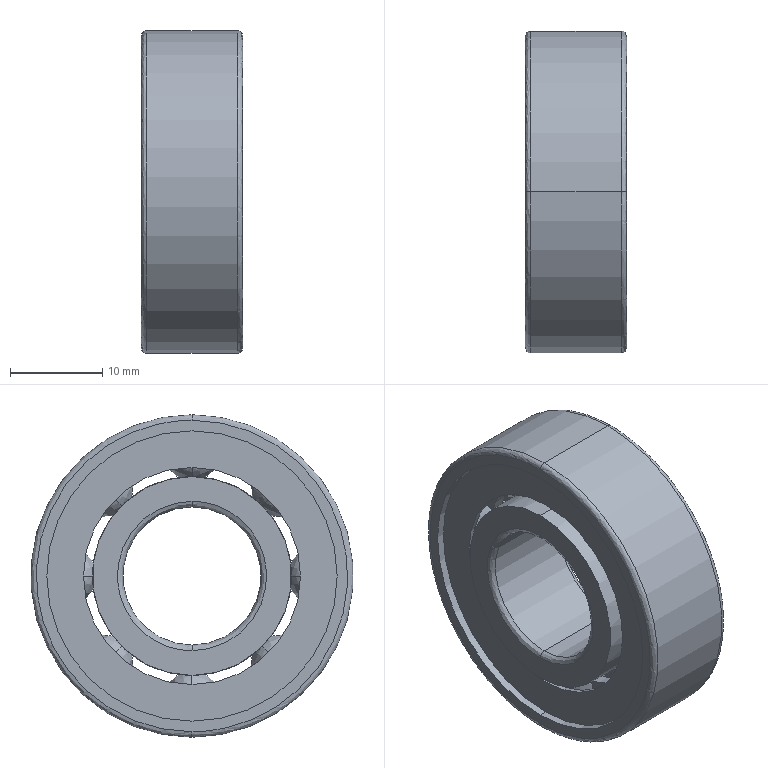Part | STEP file | 1 solid | 136 faces | box 11 x 35 x 35 mm | volume 5280 mm3 | spline 88 | cylinder 24 | plane 24 | commonest cylinder face diameters 31.5 x8 21.6 x4 23.564 x4 15 x2 24.913 x2 28.187 x2